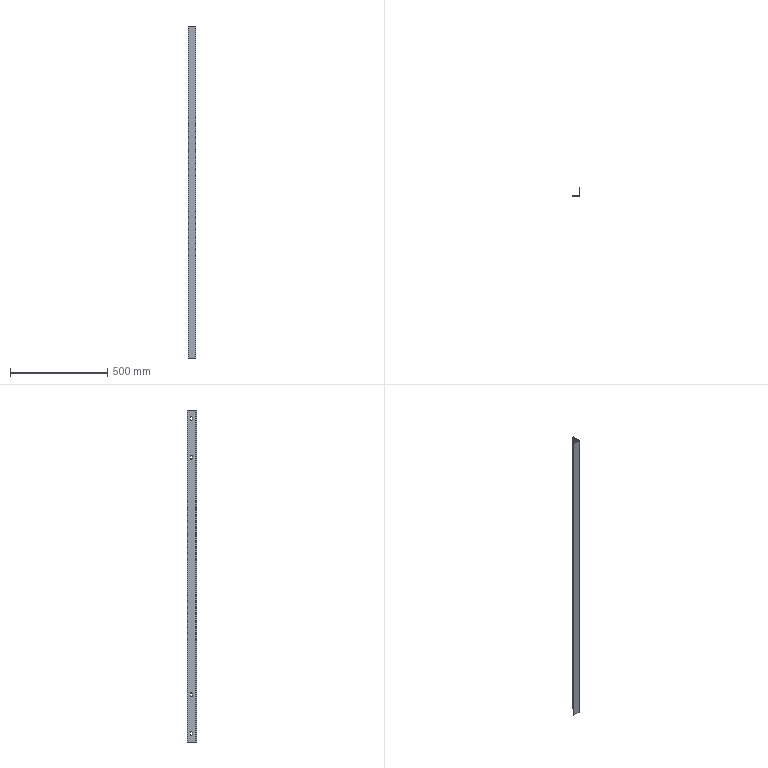Part | STEP file | SYL_0392D6J1SYL0380DJ100-519976 | 1 solid | 38 faces | box 41 x 47 x 1707 mm | volume 289245 mm3 | plane 20 | cylinder 18 | commonest cylinder face diameters 10 x16 2 x1 6 x1
STEP:
#1=CARTESIAN_POINT('',(0.,32.5,805.));
#2=VERTEX_POINT('',#1);
#3=CARTESIAN_POINT('',(-2.,32.5,805.));
#4=VERTEX_POINT('',#3);
#5=CARTESIAN_POINT('',(-2.,32.5,805.));
#6=DIRECTION('',(-1.,0.,0.));
#7=VECTOR('',#6,1000.);
#8=LINE('',#5,#7);
#9=EDGE_CURVE('',#2,#4,#8,.T.);
#10=ORIENTED_EDGE('',*,*,#9,.F.);
#11=CARTESIAN_POINT('',(0.,32.5,815.));
#12=VERTEX_POINT('',#11);
#13=CARTESIAN_POINT('',(0.,32.5,-853.5));
#14=DIRECTION('',(0.,0.,1.));
#15=VECTOR('',#14,1000.);
#16=LINE('',#13,#15);
#17=EDGE_CURVE('',#2,#12,#16,.T.);
#18=ORIENTED_EDGE('',*,*,#17,.T.);
#19=CARTESIAN_POINT('',(-2.,32.5,815.));
#20=VERTEX_POINT('',#19);
#21=CARTESIAN_POINT('',(-2.,32.5,815.));
#22=DIRECTION('',(-1.,0.,0.));
#23=VECTOR('',#22,1000.);
#24=LINE('',#21,#23);
#25=EDGE_CURVE('',#12,#20,#24,.T.);
#26=ORIENTED_EDGE('',*,*,#25,.T.);
#27=CARTESIAN_POINT('',(-2.,32.5,805.));
#28=DIRECTION('',(0.,0.,1.));
#29=VECTOR('',#28,1000.);
#30=LINE('',#27,#29);
#31=EDGE_CURVE('',#4,#20,#30,.T.);
#32=ORIENTED_EDGE('',*,*,#31,.F.);
#33=EDGE_LOOP('',(#10,#18,#26,#32));
#34=FACE_OUTER_BOUND('',#33,.T.);
#35=CARTESIAN_POINT('',(-2.,32.5,805.));
#36=DIRECTION('',(0.,1.,0.));
#37=DIRECTION('',(0.,0.,1.));
#38=AXIS2_PLACEMENT_3D('',#35,#36,#37);
#39=PLANE('',#38);
#40=ADVANCED_FACE('',(#34),#39,.F.);
#41=ORIENTED_EDGE('',*,*,#25,.F.);
#42=CARTESIAN_POINT('',(0.,27.5,820.));
#43=VERTEX_POINT('',#42);
#44=CARTESIAN_POINT('',(0.,27.5,815.));
#45=DIRECTION('',(1.,0.,0.));
#46=DIRECTION('',(0.,0.,-1.));
#47=AXIS2_PLACEMENT_3D('',#44,#45,#46);
#48=CIRCLE('',#47,5.);
#49=EDGE_CURVE('',#12,#43,#48,.T.);
#50=ORIENTED_EDGE('',*,*,#49,.T.);
#51=CARTESIAN_POINT('',(-2.,27.5,820.));
#52=VERTEX_POINT('',#51);
#53=CARTESIAN_POINT('',(-2.,27.5,820.));
#54=DIRECTION('',(-1.,0.,0.));
#55=VECTOR('',#54,1000.);
#56=LINE('',#53,#55);
#57=EDGE_CURVE('',#43,#52,#56,.T.);
#58=ORIENTED_EDGE('',*,*,#57,.T.);
#59=CARTESIAN_POINT('',(-2.,27.5,815.));
#60=DIRECTION('',(1.,0.,0.));
#61=DIRECTION('',(0.,1.,0.));
#62=AXIS2_PLACEMENT_3D('',#59,#60,#61);
#63=CIRCLE('',#62,5.);
#64=EDGE_CURVE('',#20,#52,#63,.T.);
#65=ORIENTED_EDGE('',*,*,#64,.F.);
#66=EDGE_LOOP('',(#41,#50,#58,#65));
#67=FACE_OUTER_BOUND('',#66,.T.);
#68=CARTESIAN_POINT('',(-2.,27.5,815.));
#69=DIRECTION('',(1.,0.,0.));
#70=DIRECTION('',(0.,0.,-1.));
#71=AXIS2_PLACEMENT_3D('',#68,#69,#70);
#72=CYLINDRICAL_SURFACE('',#71,5.);
#73=ADVANCED_FACE('',(#67),#72,.F.);
#74=ORIENTED_EDGE('',*,*,#57,.F.);
#75=CARTESIAN_POINT('',(0.,22.5,815.));
#76=VERTEX_POINT('',#75);
#77=CARTESIAN_POINT('',(0.,27.5,815.));
#78=DIRECTION('',(1.,0.,0.));
#79=DIRECTION('',(0.,0.,-1.));
#80=AXIS2_PLACEMENT_3D('',#77,#78,#79);
#81=CIRCLE('',#80,5.);
#82=EDGE_CURVE('',#43,#76,#81,.T.);
#83=ORIENTED_EDGE('',*,*,#82,.T.);
#84=CARTESIAN_POINT('',(-2.,22.5,815.));
#85=VERTEX_POINT('',#84);
#86=CARTESIAN_POINT('',(-2.,22.5,815.));
#87=DIRECTION('',(-1.,0.,0.));
#88=VECTOR('',#87,1000.);
#89=LINE('',#86,#88);
#90=EDGE_CURVE('',#76,#85,#89,.T.);
#91=ORIENTED_EDGE('',*,*,#90,.T.);
#92=CARTESIAN_POINT('',(-2.,27.5,815.));
#93=DIRECTION('',(1.,0.,0.));
#94=DIRECTION('',(0.,0.,1.));
#95=AXIS2_PLACEMENT_3D('',#92,#93,#94);
#96=CIRCLE('',#95,5.);
#97=EDGE_CURVE('',#52,#85,#96,.T.);
#98=ORIENTED_EDGE('',*,*,#97,.F.);
#99=EDGE_LOOP('',(#74,#83,#91,#98));
#100=FACE_OUTER_BOUND('',#99,.T.);
#101=CARTESIAN_POINT('',(-2.,27.5,815.));
#102=DIRECTION('',(1.,0.,0.));
#103=DIRECTION('',(0.,0.,-1.));
#104=AXIS2_PLACEMENT_3D('',#101,#102,#103);
#105=CYLINDRICAL_SURFACE('',#104,5.);
#106=ADVANCED_FACE('',(#100),#105,.F.);
#107=ORIENTED_EDGE('',*,*,#90,.F.);
#108=CARTESIAN_POINT('',(0.,22.5,805.));
#109=VERTEX_POINT('',#108);
#110=CARTESIAN_POINT('',(0.,22.5,-853.5));
#111=DIRECTION('',(0.,0.,-1.));
#112=VECTOR('',#111,1000.);
#113=LINE('',#110,#112);
#114=EDGE_CURVE('',#76,#109,#113,.T.);
#115=ORIENTED_EDGE('',*,*,#114,.T.);
#116=CARTESIAN_POINT('',(-2.,22.5,805.));
#117=VERTEX_POINT('',#116);
#118=CARTESIAN_POINT('',(-2.,22.5,805.));
#119=DIRECTION('',(-1.,0.,0.));
#120=VECTOR('',#119,1000.);
#121=LINE('',#118,#120);
#122=EDGE_CURVE('',#109,#117,#121,.T.);
#123=ORIENTED_EDGE('',*,*,#122,.T.);
#124=CARTESIAN_POINT('',(-2.,22.5,815.));
#125=DIRECTION('',(0.,0.,-1.));
#126=VECTOR('',#125,1000.);
#127=LINE('',#124,#126);
#128=EDGE_CURVE('',#85,#117,#127,.T.);
#129=ORIENTED_EDGE('',*,*,#128,.F.);
#130=EDGE_LOOP('',(#107,#115,#123,#129));
#131=FACE_OUTER_BOUND('',#130,.T.);
#132=CARTESIAN_POINT('',(-2.,22.5,815.));
#133=DIRECTION('',(0.,-1.,0.));
#134=DIRECTION('',(0.,0.,-1.));
#135=AXIS2_PLACEMENT_3D('',#132,#133,#134);
#136=PLANE('',#135);
#137=ADVANCED_FACE('',(#131),#136,.F.);
#138=ORIENTED_EDGE('',*,*,#122,.F.);
#139=CARTESIAN_POINT('',(0.,27.5,800.));
#140=VERTEX_POINT('',#139);
#141=CARTESIAN_POINT('',(0.,27.5,805.));
#142=DIRECTION('',(1.,0.,0.));
#143=DIRECTION('',(0.,0.,-1.));
#144=AXIS2_PLACEMENT_3D('',#141,#142,#143);
#145=CIRCLE('',#144,5.);
#146=EDGE_CURVE('',#109,#140,#145,.T.);
#147=ORIENTED_EDGE('',*,*,#146,.T.);
#148=CARTESIAN_POINT('',(-2.,27.5,800.));
#149=VERTEX_POINT('',#148);
#150=CARTESIAN_POINT('',(-2.,27.5,800.));
#151=DIRECTION('',(-1.,0.,0.));
#152=VECTOR('',#151,1000.);
#153=LINE('',#150,#152);
#154=EDGE_CURVE('',#140,#149,#153,.T.);
#155=ORIENTED_EDGE('',*,*,#154,.T.);
#156=CARTESIAN_POINT('',(-2.,27.5,805.));
#157=DIRECTION('',(1.,0.,0.));
#158=DIRECTION('',(0.,-1.,0.));
#159=AXIS2_PLACEMENT_3D('',#156,#157,#158);
#160=CIRCLE('',#159,5.);
#161=EDGE_CURVE('',#117,#149,#160,.T.);
#162=ORIENTED_EDGE('',*,*,#161,.F.);
#163=EDGE_LOOP('',(#138,#147,#155,#162));
#164=FACE_OUTER_BOUND('',#163,.T.);
#165=CARTESIAN_POINT('',(-2.,27.5,805.));
#166=DIRECTION('',(1.,0.,0.));
#167=DIRECTION('',(0.,0.,-1.));
#168=AXIS2_PLACEMENT_3D('',#165,#166,#167);
#169=CYLINDRICAL_SURFACE('',#168,5.);
#170=ADVANCED_FACE('',(#164),#169,.F.);
#171=CARTESIAN_POINT('',(0.,32.5,605.));
#172=VERTEX_POINT('',#171);
#173=CARTESIAN_POINT('',(-2.,32.5,605.));
#174=VERTEX_POINT('',#173);
#175=CARTESIAN_POINT('',(-2.,32.5,605.));
#176=DIRECTION('',(-1.,0.,0.));
#177=VECTOR('',#176,1000.);
#178=LINE('',#175,#177);
#179=EDGE_CURVE('',#172,#174,#178,.T.);
#180=ORIENTED_EDGE('',*,*,#179,.F.);
#181=CARTESIAN_POINT('',(0.,32.5,615.));
#182=VERTEX_POINT('',#181);
#183=CARTESIAN_POINT('',(0.,32.5,-853.5));
#184=DIRECTION('',(0.,0.,1.));
#185=VECTOR('',#184,1000.);
#186=LINE('',#183,#185);
#187=EDGE_CURVE('',#172,#182,#186,.T.);
#188=ORIENTED_EDGE('',*,*,#187,.T.);
#189=CARTESIAN_POINT('',(-2.,32.5,615.));
#190=VERTEX_POINT('',#189);
#191=CARTESIAN_POINT('',(-2.,32.5,615.));
#192=DIRECTION('',(-1.,0.,0.));
#193=VECTOR('',#192,1000.);
#194=LINE('',#191,#193);
#195=EDGE_CURVE('',#182,#190,#194,.T.);
#196=ORIENTED_EDGE('',*,*,#195,.T.);
#197=CARTESIAN_POINT('',(-2.,32.5,605.));
#198=DIRECTION('',(0.,0.,1.));
#199=VECTOR('',#198,1000.);
#200=LINE('',#197,#199);
#201=EDGE_CURVE('',#174,#190,#200,.T.);
#202=ORIENTED_EDGE('',*,*,#201,.F.);
#203=EDGE_LOOP('',(#180,#188,#196,#202));
#204=FACE_OUTER_BOUND('',#203,.T.);
#205=CARTESIAN_POINT('',(-2.,32.5,605.));
#206=DIRECTION('',(0.,1.,0.));
#207=DIRECTION('',(0.,0.,1.));
#208=AXIS2_PLACEMENT_3D('',#205,#206,#207);
#209=PLANE('',#208);
#210=ADVANCED_FACE('',(#204),#209,.F.);
#211=ORIENTED_EDGE('',*,*,#195,.F.);
#212=CARTESIAN_POINT('',(0.,27.5,620.));
#213=VERTEX_POINT('',#212);
#214=CARTESIAN_POINT('',(0.,27.5,615.));
#215=DIRECTION('',(1.,0.,0.));
#216=DIRECTION('',(0.,0.,-1.));
#217=AXIS2_PLACEMENT_3D('',#214,#215,#216);
#218=CIRCLE('',#217,5.);
#219=EDGE_CURVE('',#182,#213,#218,.T.);
#220=ORIENTED_EDGE('',*,*,#219,.T.);
#221=CARTESIAN_POINT('',(-2.,27.5,620.));
#222=VERTEX_POINT('',#221);
#223=CARTESIAN_POINT('',(-2.,27.5,620.));
#224=DIRECTION('',(-1.,0.,0.));
#225=VECTOR('',#224,1000.);
#226=LINE('',#223,#225);
#227=EDGE_CURVE('',#213,#222,#226,.T.);
#228=ORIENTED_EDGE('',*,*,#227,.T.);
#229=CARTESIAN_POINT('',(-2.,27.5,615.));
#230=DIRECTION('',(1.,0.,0.));
#231=DIRECTION('',(0.,1.,0.));
#232=AXIS2_PLACEMENT_3D('',#229,#230,#231);
#233=CIRCLE('',#232,5.);
#234=EDGE_CURVE('',#190,#222,#233,.T.);
#235=ORIENTED_EDGE('',*,*,#234,.F.);
#236=EDGE_LOOP('',(#211,#220,#228,#235));
#237=FACE_OUTER_BOUND('',#236,.T.);
#238=CARTESIAN_POINT('',(-2.,27.5,615.));
#239=DIRECTION('',(1.,0.,0.));
#240=DIRECTION('',(0.,0.,-1.));
#241=AXIS2_PLACEMENT_3D('',#238,#239,#240);
#242=CYLINDRICAL_SURFACE('',#241,5.);
#243=ADVANCED_FACE('',(#237),#242,.F.);
#244=ORIENTED_EDGE('',*,*,#227,.F.);
#245=CARTESIAN_POINT('',(0.,22.5,615.));
#246=VERTEX_POINT('',#245);
#247=CARTESIAN_POINT('',(0.,27.5,615.));
#248=DIRECTION('',(1.,0.,0.));
#249=DIRECTION('',(0.,0.,-1.));
#250=AXIS2_PLACEMENT_3D('',#247,#248,#249);
#251=CIRCLE('',#250,5.);
#252=EDGE_CURVE('',#213,#246,#251,.T.);
#253=ORIENTED_EDGE('',*,*,#252,.T.);
#254=CARTESIAN_POINT('',(-2.,22.5,615.));
#255=VERTEX_POINT('',#254);
#256=CARTESIAN_POINT('',(-2.,22.5,615.));
#257=DIRECTION('',(-1.,0.,0.));
#258=VECTOR('',#257,1000.);
#259=LINE('',#256,#258);
#260=EDGE_CURVE('',#246,#255,#259,.T.);
#261=ORIENTED_EDGE('',*,*,#260,.T.);
#262=CARTESIAN_POINT('',(-2.,27.5,615.));
#263=DIRECTION('',(1.,0.,0.));
#264=DIRECTION('',(0.,0.,1.));
#265=AXIS2_PLACEMENT_3D('',#262,#263,#264);
#266=CIRCLE('',#265,5.);
#267=EDGE_CURVE('',#222,#255,#266,.T.);
#268=ORIENTED_EDGE('',*,*,#267,.F.);
#269=EDGE_LOOP('',(#244,#253,#261,#268));
#270=FACE_OUTER_BOUND('',#269,.T.);
#271=CARTESIAN_POINT('',(-2.,27.5,615.));
#272=DIRECTION('',(1.,0.,0.));
#273=DIRECTION('',(0.,0.,-1.));
#274=AXIS2_PLACEMENT_3D('',#271,#272,#273);
#275=CYLINDRICAL_SURFACE('',#274,5.);
#276=ADVANCED_FACE('',(#270),#275,.F.);
#277=ORIENTED_EDGE('',*,*,#260,.F.);
#278=CARTESIAN_POINT('',(0.,22.5,605.));
#279=VERTEX_POINT('',#278);
#280=CARTESIAN_POINT('',(0.,22.5,-853.5));
#281=DIRECTION('',(0.,0.,-1.));
#282=VECTOR('',#281,1000.);
#283=LINE('',#280,#282);
#284=EDGE_CURVE('',#246,#279,#283,.T.);
#285=ORIENTED_EDGE('',*,*,#284,.T.);
#286=CARTESIAN_POINT('',(-2.,22.5,605.));
#287=VERTEX_POINT('',#286);
#288=CARTESIAN_POINT('',(-2.,22.5,605.));
#289=DIRECTION('',(-1.,0.,0.));
#290=VECTOR('',#289,1000.);
#291=LINE('',#288,#290);
#292=EDGE_CURVE('',#279,#287,#291,.T.);
#293=ORIENTED_EDGE('',*,*,#292,.T.);
#294=CARTESIAN_POINT('',(-2.,22.5,615.));
#295=DIRECTION('',(0.,0.,-1.));
#296=VECTOR('',#295,1000.);
#297=LINE('',#294,#296);
#298=EDGE_CURVE('',#255,#287,#297,.T.);
#299=ORIENTED_EDGE('',*,*,#298,.F.);
#300=EDGE_LOOP('',(#277,#285,#293,#299));
#301=FACE_OUTER_BOUND('',#300,.T.);
#302=CARTESIAN_POINT('',(-2.,22.5,615.));
#303=DIRECTION('',(0.,-1.,0.));
#304=DIRECTION('',(0.,0.,-1.));
#305=AXIS2_PLACEMENT_3D('',#302,#303,#304);
#306=PLANE('',#305);
#307=ADVANCED_FACE('',(#301),#306,.F.);
#308=ORIENTED_EDGE('',*,*,#292,.F.);
#309=CARTESIAN_POINT('',(0.,27.5,600.));
#310=VERTEX_POINT('',#309);
#311=CARTESIAN_POINT('',(0.,27.5,605.));
#312=DIRECTION('',(1.,0.,0.));
#313=DIRECTION('',(0.,0.,-1.));
#314=AXIS2_PLACEMENT_3D('',#311,#312,#313);
#315=CIRCLE('',#314,5.);
#316=EDGE_CURVE('',#279,#310,#315,.T.);
#317=ORIENTED_EDGE('',*,*,#316,.T.);
#318=CARTESIAN_POINT('',(-2.,27.5,600.));
#319=VERTEX_POINT('',#318);
#320=CARTESIAN_POINT('',(-2.,27.5,600.));
#321=DIRECTION('',(-1.,0.,0.));
#322=VECTOR('',#321,1000.);
#323=LINE('',#320,#322);
#324=EDGE_CURVE('',#310,#319,#323,.T.);
#325=ORIENTED_EDGE('',*,*,#324,.T.);
#326=CARTESIAN_POINT('',(-2.,27.5,605.));
#327=DIRECTION('',(1.,0.,0.));
#328=DIRECTION('',(0.,-1.,0.));
#329=AXIS2_PLACEMENT_3D('',#326,#327,#328);
#330=CIRCLE('',#329,5.);
#331=EDGE_CURVE('',#287,#319,#330,.T.);
#332=ORIENTED_EDGE('',*,*,#331,.F.);
#333=EDGE_LOOP('',(#308,#317,#325,#332));
#334=FACE_OUTER_BOUND('',#333,.T.);
#335=CARTESIAN_POINT('',(-2.,27.5,605.));
#336=DIRECTION('',(1.,0.,0.));
#337=DIRECTION('',(0.,0.,-1.));
#338=AXIS2_PLACEMENT_3D('',#335,#336,#337);
#339=CYLINDRICAL_SURFACE('',#338,5.);
#340=ADVANCED_FACE('',(#334),#339,.F.);
#341=CARTESIAN_POINT('',(0.,32.5,-815.));
#342=VERTEX_POINT('',#341);
#343=CARTESIAN_POINT('',(-2.,32.5,-815.));
#344=VERTEX_POINT('',#343);
#345=CARTESIAN_POINT('',(-2.,32.5,-815.));
#346=DIRECTION('',(-1.,0.,0.));
#347=VECTOR('',#346,1000.);
#348=LINE('',#345,#347);
#349=EDGE_CURVE('',#342,#344,#348,.T.);
#350=ORIENTED_EDGE('',*,*,#349,.F.);
#351=CARTESIAN_POINT('',(0.,32.5,-805.));
#352=VERTEX_POINT('',#351);
#353=CARTESIAN_POINT('',(0.,32.5,-853.5));
#354=DIRECTION('',(0.,0.,-1.));
#355=VECTOR('',#354,1000.);
#356=LINE('',#353,#355);
#357=EDGE_CURVE('',#352,#342,#356,.T.);
#358=ORIENTED_EDGE('',*,*,#357,.F.);
#359=CARTESIAN_POINT('',(-2.,32.5,-805.));
#360=VERTEX_POINT('',#359);
#361=CARTESIAN_POINT('',(-2.,32.5,-805.));
#362=DIRECTION('',(-1.,0.,0.));
#363=VECTOR('',#362,1000.);
#364=LINE('',#361,#363);
#365=EDGE_CURVE('',#352,#360,#364,.T.);
#366=ORIENTED_EDGE('',*,*,#365,.T.);
#367=CARTESIAN_POINT('',(-2.,32.5,-805.));
#368=DIRECTION('',(0.,0.,-1.));
#369=VECTOR('',#368,1000.);
#370=LINE('',#367,#369);
#371=EDGE_CURVE('',#360,#344,#370,.T.);
#372=ORIENTED_EDGE('',*,*,#371,.T.);
#373=EDGE_LOOP('',(#350,#358,#366,#372));
#374=FACE_OUTER_BOUND('',#373,.T.);
#375=CARTESIAN_POINT('',(-2.,32.5,-805.));
#376=DIRECTION('',(0.,-1.,0.));
#377=DIRECTION('',(0.,0.,-1.));
#378=AXIS2_PLACEMENT_3D('',#375,#376,#377);
#379=PLANE('',#378);
#380=ADVANCED_FACE('',(#374),#379,.T.);
#381=ORIENTED_EDGE('',*,*,#365,.F.);
#382=CARTESIAN_POINT('',(0.,27.5,-800.));
#383=VERTEX_POINT('',#382);
#384=CARTESIAN_POINT('',(0.,27.5,-805.));
#385=DIRECTION('',(1.,0.,0.));
#386=DIRECTION('',(0.,0.,-1.));
#387=AXIS2_PLACEMENT_3D('',#384,#385,#386);
#388=CIRCLE('',#387,5.);
#389=EDGE_CURVE('',#352,#383,#388,.T.);
#390=ORIENTED_EDGE('',*,*,#389,.T.);
#391=CARTESIAN_POINT('',(-2.,27.5,-800.));
#392=VERTEX_POINT('',#391);
#393=CARTESIAN_POINT('',(-2.,27.5,-800.));
#394=DIRECTION('',(-1.,0.,0.));
#395=VECTOR('',#394,1000.);
#396=LINE('',#393,#395);
#397=EDGE_CURVE('',#383,#392,#396,.T.);
#398=ORIENTED_EDGE('',*,*,#397,.T.);
#399=CARTESIAN_POINT('',(-2.,27.5,-805.));
#400=DIRECTION('',(1.,0.,0.));
#401=DIRECTION('',(0.,1.,0.));
#402=AXIS2_PLACEMENT_3D('',#399,#400,#401);
#403=CIRCLE('',#402,5.);
#404=EDGE_CURVE('',#360,#392,#403,.T.);
#405=ORIENTED_EDGE('',*,*,#404,.F.);
#406=EDGE_LOOP('',(#381,#390,#398,#405));
#407=FACE_OUTER_BOUND('',#406,.T.);
#408=CARTESIAN_POINT('',(-2.,27.5,-805.));
#409=DIRECTION('',(1.,0.,0.));
#410=DIRECTION('',(0.,0.,-1.));
#411=AXIS2_PLACEMENT_3D('',#408,#409,#410);
#412=CYLINDRICAL_SURFACE('',#411,5.);
#413=ADVANCED_FACE('',(#407),#412,.F.);
#414=ORIENTED_EDGE('',*,*,#397,.F.);
#415=CARTESIAN_POINT('',(0.,22.5,-805.));
#416=VERTEX_POINT('',#415);
#417=CARTESIAN_POINT('',(0.,27.5,-805.));
#418=DIRECTION('',(1.,0.,0.));
#419=DIRECTION('',(0.,0.,-1.));
#420=AXIS2_PLACEMENT_3D('',#417,#418,#419);
#421=CIRCLE('',#420,5.);
#422=EDGE_CURVE('',#383,#416,#421,.T.);
#423=ORIENTED_EDGE('',*,*,#422,.T.);
#424=CARTESIAN_POINT('',(-2.,22.5,-805.));
#425=VERTEX_POINT('',#424);
#426=CARTESIAN_POINT('',(-2.,22.5,-805.));
#427=DIRECTION('',(-1.,0.,0.));
#428=VECTOR('',#427,1000.);
#429=LINE('',#426,#428);
#430=EDGE_CURVE('',#416,#425,#429,.T.);
#431=ORIENTED_EDGE('',*,*,#430,.T.);
#432=CARTESIAN_POINT('',(-2.,27.5,-805.));
#433=DIRECTION('',(1.,0.,0.));
#434=DIRECTION('',(0.,0.,1.));
#435=AXIS2_PLACEMENT_3D('',#432,#433,#434);
#436=CIRCLE('',#435,5.);
#437=EDGE_CURVE('',#392,#425,#436,.T.);
#438=ORIENTED_EDGE('',*,*,#437,.F.);
#439=EDGE_LOOP('',(#414,#423,#431,#438));
#440=FACE_OUTER_BOUND('',#439,.T.);
#441=CARTESIAN_POINT('',(-2.,27.5,-805.));
#442=DIRECTION('',(1.,0.,0.));
#443=DIRECTION('',(0.,0.,-1.));
#444=AXIS2_PLACEMENT_3D('',#441,#442,#443);
#445=CYLINDRICAL_SURFACE('',#444,5.);
#446=ADVANCED_FACE('',(#440),#445,.F.);
#447=ORIENTED_EDGE('',*,*,#430,.F.);
#448=CARTESIAN_POINT('',(0.,22.5,-815.));
#449=VERTEX_POINT('',#448);
#450=CARTESIAN_POINT('',(0.,22.5,-853.5));
#451=DIRECTION('',(0.,0.,1.));
#452=VECTOR('',#451,1000.);
#453=LINE('',#450,#452);
#454=EDGE_CURVE('',#449,#416,#453,.T.);
#455=ORIENTED_EDGE('',*,*,#454,.F.);
#456=CARTESIAN_POINT('',(-2.,22.5,-815.));
#457=VERTEX_POINT('',#456);
#458=CARTESIAN_POINT('',(-2.,22.5,-815.));
#459=DIRECTION('',(-1.,0.,0.));
#460=VECTOR('',#459,1000.);
#461=LINE('',#458,#460);
#462=EDGE_CURVE('',#449,#457,#461,.T.);
#463=ORIENTED_EDGE('',*,*,#462,.T.);
#464=CARTESIAN_POINT('',(-2.,22.5,-815.));
#465=DIRECTION('',(0.,0.,1.));
#466=VECTOR('',#465,1000.);
#467=LINE('',#464,#466);
#468=EDGE_CURVE('',#457,#425,#467,.T.);
#469=ORIENTED_EDGE('',*,*,#468,.T.);
#470=EDGE_LOOP('',(#447,#455,#463,#469));
#471=FACE_OUTER_BOUND('',#470,.T.);
#472=CARTESIAN_POINT('',(-2.,22.5,-815.));
#473=DIRECTION('',(0.,1.,0.));
#474=DIRECTION('',(0.,0.,1.));
#475=AXIS2_PLACEMENT_3D('',#472,#473,#474);
#476=PLANE('',#475);
#477=ADVANCED_FACE('',(#471),#476,.T.);
#478=ORIENTED_EDGE('',*,*,#462,.F.);
#479=CARTESIAN_POINT('',(0.,27.5,-820.));
#480=VERTEX_POINT('',#479);
#481=CARTESIAN_POINT('',(0.,27.5,-815.));
#482=DIRECTION('',(1.,0.,0.));
#483=DIRECTION('',(0.,0.,-1.));
#484=AXIS2_PLACEMENT_3D('',#481,#482,#483);
#485=CIRCLE('',#484,5.);
#486=EDGE_CURVE('',#449,#480,#485,.T.);
#487=ORIENTED_EDGE('',*,*,#486,.T.);
#488=CARTESIAN_POINT('',(-2.,27.5,-820.));
#489=VERTEX_POINT('',#488);
#490=CARTESIAN_POINT('',(-2.,27.5,-820.));
#491=DIRECTION('',(-1.,0.,0.));
#492=VECTOR('',#491,1000.);
#493=LINE('',#490,#492);
#494=EDGE_CURVE('',#480,#489,#493,.T.);
#495=ORIENTED_EDGE('',*,*,#494,.T.);
#496=CARTESIAN_POINT('',(-2.,27.5,-815.));
#497=DIRECTION('',(1.,0.,0.));
#498=DIRECTION('',(0.,-1.,0.));
#499=AXIS2_PLACEMENT_3D('',#496,#497,#498);
#500=CIRCLE('',#499,5.);
#501=EDGE_CURVE('',#457,#489,#500,.T.);
#502=ORIENTED_EDGE('',*,*,#501,.F.);
#503=EDGE_LOOP('',(#478,#487,#495,#502));
#504=FACE_OUTER_BOUND('',#503,.T.);
#505=CARTESIAN_POINT('',(-2.,27.5,-815.));
#506=DIRECTION('',(1.,0.,0.));
#507=DIRECTION('',(0.,0.,-1.));
#508=AXIS2_PLACEMENT_3D('',#505,#506,#507);
#509=CYLINDRICAL_SURFACE('',#508,5.);
#510=ADVANCED_FACE('',(#504),#509,.F.);
#511=CARTESIAN_POINT('',(0.,32.5,-615.));
#512=VERTEX_POINT('',#511);
#513=CARTESIAN_POINT('',(-2.,32.5,-615.));
#514=VERTEX_POINT('',#513);
#515=CARTESIAN_POINT('',(-2.,32.5,-615.));
#516=DIRECTION('',(-1.,0.,0.));
#517=VECTOR('',#516,1000.);
#518=LINE('',#515,#517);
#519=EDGE_CURVE('',#512,#514,#518,.T.);
#520=ORIENTED_EDGE('',*,*,#519,.F.);
#521=CARTESIAN_POINT('',(0.,32.5,-605.));
#522=VERTEX_POINT('',#521);
#523=CARTESIAN_POINT('',(0.,32.5,-853.5));
#524=DIRECTION('',(0.,0.,-1.));
#525=VECTOR('',#524,1000.);
#526=LINE('',#523,#525);
#527=EDGE_CURVE('',#522,#512,#526,.T.);
#528=ORIENTED_EDGE('',*,*,#527,.F.);
#529=CARTESIAN_POINT('',(-2.,32.5,-605.));
#530=VERTEX_POINT('',#529);
#531=CARTESIAN_POINT('',(-2.,32.5,-605.));
#532=DIRECTION('',(-1.,0.,0.));
#533=VECTOR('',#532,1000.);
#534=LINE('',#531,#533);
#535=EDGE_CURVE('',#522,#530,#534,.T.);
#536=ORIENTED_EDGE('',*,*,#535,.T.);
#537=CARTESIAN_POINT('',(-2.,32.5,-605.));
#538=DIRECTION('',(0.,0.,-1.));
#539=VECTOR('',#538,1000.);
#540=LINE('',#537,#539);
#541=EDGE_CURVE('',#530,#514,#540,.T.);
#542=ORIENTED_EDGE('',*,*,#541,.T.);
#543=EDGE_LOOP('',(#520,#528,#536,#542));
#544=FACE_OUTER_BOUND('',#543,.T.);
#545=CARTESIAN_POINT('',(-2.,32.5,-605.));
#546=DIRECTION('',(0.,-1.,0.));
#547=DIRECTION('',(0.,0.,-1.));
#548=AXIS2_PLACEMENT_3D('',#545,#546,#547);
#549=PLANE('',#548);
#550=ADVANCED_FACE('',(#544),#549,.T.);
#551=ORIENTED_EDGE('',*,*,#535,.F.);
#552=CARTESIAN_POINT('',(0.,27.5,-600.));
#553=VERTEX_POINT('',#552);
#554=CARTESIAN_POINT('',(0.,27.5,-605.));
#555=DIRECTION('',(1.,0.,0.));
#556=DIRECTION('',(0.,0.,-1.));
#557=AXIS2_PLACEMENT_3D('',#554,#555,#556);
#558=CIRCLE('',#557,5.);
#559=EDGE_CURVE('',#522,#553,#558,.T.);
#560=ORIENTED_EDGE('',*,*,#559,.T.);
#561=CARTESIAN_POINT('',(-2.,27.5,-600.));
#562=VERTEX_POINT('',#561);
#563=CARTESIAN_POINT('',(-2.,27.5,-600.));
#564=DIRECTION('',(-1.,0.,0.));
#565=VECTOR('',#564,1000.);
#566=LINE('',#563,#565);
#567=EDGE_CURVE('',#553,#562,#566,.T.);
#568=ORIENTED_EDGE('',*,*,#567,.T.);
#569=CARTESIAN_POINT('',(-2.,27.5,-605.));
#570=DIRECTION('',(1.,0.,0.));
#571=DIRECTION('',(0.,1.,0.));
#572=AXIS2_PLACEMENT_3D('',#569,#570,#571);
#573=CIRCLE('',#572,5.);
#574=EDGE_CURVE('',#530,#562,#573,.T.);
#575=ORIENTED_EDGE('',*,*,#574,.F.);
#576=EDGE_LOOP('',(#551,#560,#568,#575));
#577=FACE_OUTER_BOUND('',#576,.T.);
#578=CARTESIAN_POINT('',(-2.,27.5,-605.));
#579=DIRECTION('',(1.,0.,0.));
#580=DIRECTION('',(0.,0.,-1.));
#581=AXIS2_PLACEMENT_3D('',#578,#579,#580);
#582=CYLINDRICAL_SURFACE('',#581,5.);
#583=ADVANCED_FACE('',(#577),#582,.F.);
#584=ORIENTED_EDGE('',*,*,#567,.F.);
#585=CARTESIAN_POINT('',(0.,22.5,-605.));
#586=VERTEX_POINT('',#585);
#587=CARTESIAN_POINT('',(0.,27.5,-605.));
#588=DIRECTION('',(1.,0.,0.));
#589=DIRECTION('',(0.,0.,-1.));
#590=AXIS2_PLACEMENT_3D('',#587,#588,#589);
#591=CIRCLE('',#590,5.);
#592=EDGE_CURVE('',#553,#586,#591,.T.);
#593=ORIENTED_EDGE('',*,*,#592,.T.);
#594=CARTESIAN_POINT('',(-2.,22.5,-605.));
#595=VERTEX_POINT('',#594);
#596=CARTESIAN_POINT('',(-2.,22.5,-605.));
#597=DIRECTION('',(-1.,0.,0.));
#598=VECTOR('',#597,1000.);
#599=LINE('',#596,#598);
#600=EDGE_CURVE('',#586,#595,#599,.T.);
#601=ORIENTED_EDGE('',*,*,#600,.T.);
#602=CARTESIAN_POINT('',(-2.,27.5,-605.));
#603=DIRECTION('',(1.,0.,0.));
#604=DIRECTION('',(0.,0.,1.));
#605=AXIS2_PLACEMENT_3D('',#602,#603,#604);
#606=CIRCLE('',#605,5.);
#607=EDGE_CURVE('',#562,#595,#606,.T.);
#608=ORIENTED_EDGE('',*,*,#607,.F.);
#609=EDGE_LOOP('',(#584,#593,#601,#608));
#610=FACE_OUTER_BOUND('',#609,.T.);
#611=CARTESIAN_POINT('',(-2.,27.5,-605.));
#612=DIRECTION('',(1.,0.,0.));
#613=DIRECTION('',(0.,0.,-1.));
#614=AXIS2_PLACEMENT_3D('',#611,#612,#613);
#615=CYLINDRICAL_SURFACE('',#614,5.);
#616=ADVANCED_FACE('',(#610),#615,.F.);
#617=ORIENTED_EDGE('',*,*,#600,.F.);
#618=CARTESIAN_POINT('',(0.,22.5,-615.));
#619=VERTEX_POINT('',#618);
#620=CARTESIAN_POINT('',(0.,22.5,-853.5));
#621=DIRECTION('',(0.,0.,1.));
#622=VECTOR('',#621,1000.);
#623=LINE('',#620,#622);
#624=EDGE_CURVE('',#619,#586,#623,.T.);
#625=ORIENTED_EDGE('',*,*,#624,.F.);
#626=CARTESIAN_POINT('',(-2.,22.5,-615.));
#627=VERTEX_POINT('',#626);
#628=CARTESIAN_POINT('',(-2.,22.5,-615.));
#629=DIRECTION('',(-1.,0.,0.));
#630=VECTOR('',#629,1000.);
#631=LINE('',#628,#630);
#632=EDGE_CURVE('',#619,#627,#631,.T.);
#633=ORIENTED_EDGE('',*,*,#632,.T.);
#634=CARTESIAN_POINT('',(-2.,22.5,-615.));
#635=DIRECTION('',(0.,0.,1.));
#636=VECTOR('',#635,1000.);
#637=LINE('',#634,#636);
#638=EDGE_CURVE('',#627,#595,#637,.T.);
#639=ORIENTED_EDGE('',*,*,#638,.T.);
#640=EDGE_LOOP('',(#617,#625,#633,#639));
#641=FACE_OUTER_BOUND('',#640,.T.);
#642=CARTESIAN_POINT('',(-2.,22.5,-615.));
#643=DIRECTION('',(0.,1.,0.));
#644=DIRECTION('',(0.,0.,1.));
#645=AXIS2_PLACEMENT_3D('',#642,#643,#644);
#646=PLANE('',#645);
#647=ADVANCED_FACE('',(#641),#646,.T.);
#648=ORIENTED_EDGE('',*,*,#632,.F.);
#649=CARTESIAN_POINT('',(0.,27.5,-620.));
#650=VERTEX_POINT('',#649);
#651=CARTESIAN_POINT('',(0.,27.5,-615.));
#652=DIRECTION('',(1.,0.,0.));
#653=DIRECTION('',(0.,0.,-1.));
#654=AXIS2_PLACEMENT_3D('',#651,#652,#653);
#655=CIRCLE('',#654,5.);
#656=EDGE_CURVE('',#619,#650,#655,.T.);
#657=ORIENTED_EDGE('',*,*,#656,.T.);
#658=CARTESIAN_POINT('',(-2.,27.5,-620.));
#659=VERTEX_POINT('',#658);
#660=CARTESIAN_POINT('',(-2.,27.5,-620.));
#661=DIRECTION('',(-1.,0.,0.));
#662=VECTOR('',#661,1000.);
#663=LINE('',#660,#662);
#664=EDGE_CURVE('',#650,#659,#663,.T.);
#665=ORIENTED_EDGE('',*,*,#664,.T.);
#666=CARTESIAN_POINT('',(-2.,27.5,-615.));
#667=DIRECTION('',(1.,0.,0.));
#668=DIRECTION('',(0.,-1.,0.));
#669=AXIS2_PLACEMENT_3D('',#666,#667,#668);
#670=CIRCLE('',#669,5.);
#671=EDGE_CURVE('',#627,#659,#670,.T.);
#672=ORIENTED_EDGE('',*,*,#671,.F.);
#673=EDGE_LOOP('',(#648,#657,#665,#672));
#674=FACE_OUTER_BOUND('',#673,.T.);
#675=CARTESIAN_POINT('',(-2.,27.5,-615.));
#676=DIRECTION('',(1.,0.,0.));
#677=DIRECTION('',(0.,0.,-1.));
#678=AXIS2_PLACEMENT_3D('',#675,#676,#677);
#679=CYLINDRICAL_SURFACE('',#678,5.);
#680=ADVANCED_FACE('',(#674),#679,.F.);
#681=CARTESIAN_POINT('',(-41.,0.,-853.5));
#682=VERTEX_POINT('',#681);
#683=CARTESIAN_POINT('',(-41.,2.,-853.5));
#684=VERTEX_POINT('',#683);
#685=CARTESIAN_POINT('',(-41.,2.,-853.5));
#686=DIRECTION('',(0.,1.,0.));
#687=VECTOR('',#686,1000.);
#688=LINE('',#685,#687);
#689=EDGE_CURVE('',#682,#684,#688,.T.);
#690=ORIENTED_EDGE('',*,*,#689,.F.);
#691=CARTESIAN_POINT('',(-41.,0.,853.5));
#692=VERTEX_POINT('',#691);
#693=CARTESIAN_POINT('',(-41.,0.,-853.5));
#694=DIRECTION('',(0.,0.,-1.));
#695=VECTOR('',#694,1000.);
#696=LINE('',#693,#695);
#697=EDGE_CURVE('',#692,#682,#696,.T.);
#698=ORIENTED_EDGE('',*,*,#697,.F.);
#699=CARTESIAN_POINT('',(-41.,2.,853.5));
#700=VERTEX_POINT('',#699);
#701=CARTESIAN_POINT('',(-41.,2.,853.5));
#702=DIRECTION('',(0.,1.,0.));
#703=VECTOR('',#702,1000.);
#704=LINE('',#701,#703);
#705=EDGE_CURVE('',#692,#700,#704,.T.);
#706=ORIENTED_EDGE('',*,*,#705,.T.);
#707=CARTESIAN_POINT('',(-41.,2.,853.5));
#708=DIRECTION('',(0.,0.,-1.));
#709=VECTOR('',#708,1000.);
#710=LINE('',#707,#709);
#711=EDGE_CURVE('',#700,#684,#710,.T.);
#712=ORIENTED_EDGE('',*,*,#711,.T.);
#713=EDGE_LOOP('',(#690,#698,#706,#712));
#714=FACE_OUTER_BOUND('',#713,.T.);
#715=CARTESIAN_POINT('',(-41.,2.,853.5));
#716=DIRECTION('',(-1.,0.,0.));
#717=DIRECTION('',(0.,0.,-1.));
#718=AXIS2_PLACEMENT_3D('',#715,#716,#717);
#719=PLANE('',#718);
#720=ADVANCED_FACE('',(#714),#719,.T.);
#721=ORIENTED_EDGE('',*,*,#705,.F.);
#722=CARTESIAN_POINT('',(-3.,0.,853.5));
#723=VERTEX_POINT('',#722);
#724=CARTESIAN_POINT('',(-41.,0.,853.5));
#725=DIRECTION('',(-1.,0.,0.));
#726=VECTOR('',#725,1000.);
#727=LINE('',#724,#726);
#728=EDGE_CURVE('',#723,#692,#727,.T.);
#729=ORIENTED_EDGE('',*,*,#728,.F.);
#730=CARTESIAN_POINT('',(-3.,2.,853.5));
#731=VERTEX_POINT('',#730);
#732=CARTESIAN_POINT('',(-3.,2.,853.5));
#733=DIRECTION('',(0.,1.,0.));
#734=VECTOR('',#733,1000.);
#735=LINE('',#732,#734);
#736=EDGE_CURVE('',#723,#731,#735,.T.);
#737=ORIENTED_EDGE('',*,*,#736,.T.);
#738=CARTESIAN_POINT('',(-3.,2.,853.5));
#739=DIRECTION('',(-1.,0.,0.));
#740=VECTOR('',#739,1000.);
#741=LINE('',#738,#740);
#742=EDGE_CURVE('',#731,#700,#741,.T.);
#743=ORIENTED_EDGE('',*,*,#742,.T.);
#744=EDGE_LOOP('',(#721,#729,#737,#743));
#745=FACE_OUTER_BOUND('',#744,.T.);
#746=CARTESIAN_POINT('',(-3.,2.,853.5));
#747=DIRECTION('',(0.,0.,1.));
#748=DIRECTION('',(-1.,0.,0.));
#749=AXIS2_PLACEMENT_3D('',#746,#747,#748);
#750=PLANE('',#749);
#751=ADVANCED_FACE('',(#745),#750,.T.);
#752=ORIENTED_EDGE('',*,*,#736,.F.);
#753=CARTESIAN_POINT('',(0.,3.,853.5));
#754=VERTEX_POINT('',#753);
#755=CARTESIAN_POINT('',(-3.,3.,853.5));
#756=DIRECTION('',(0.,0.,-1.));
#757=DIRECTION('',(-1.,0.,0.));
#758=AXIS2_PLACEMENT_3D('',#755,#756,#757);
#759=CIRCLE('',#758,3.);
#760=EDGE_CURVE('',#754,#723,#759,.T.);
#761=ORIENTED_EDGE('',*,*,#760,.F.);
#762=CARTESIAN_POINT('',(-2.,3.,853.5));
#763=VERTEX_POINT('',#762);
#764=CARTESIAN_POINT('',(-2.,3.,853.5));
#765=DIRECTION('',(-1.,0.,0.));
#766=VECTOR('',#765,1000.);
#767=LINE('',#764,#766);
#768=EDGE_CURVE('',#754,#763,#767,.T.);
#769=ORIENTED_EDGE('',*,*,#768,.T.);
#770=CARTESIAN_POINT('',(-3.,3.,853.5));
#771=DIRECTION('',(0.,0.,-1.));
#772=DIRECTION('',(1.,0.,0.));
#773=AXIS2_PLACEMENT_3D('',#770,#771,#772);
#774=CIRCLE('',#773,1.);
#775=EDGE_CURVE('',#763,#731,#774,.T.);
#776=ORIENTED_EDGE('',*,*,#775,.T.);
#777=EDGE_LOOP('',(#752,#761,#769,#776));
#778=FACE_OUTER_BOUND('',#777,.T.);
#779=CARTESIAN_POINT('',(-3.,3.,853.5));
#780=DIRECTION('',(0.,0.,1.));
#781=DIRECTION('',(1.,0.,0.));
#782=AXIS2_PLACEMENT_3D('',#779,#780,#781);
#783=PLANE('',#782);
#784=ADVANCED_FACE('',(#778),#783,.T.);
#785=ORIENTED_EDGE('',*,*,#768,.F.);
#786=CARTESIAN_POINT('',(0.,47.,853.5));
#787=VERTEX_POINT('',#786);
#788=CARTESIAN_POINT('',(0.,0.,853.5));
#789=DIRECTION('',(0.,-1.,0.));
#790=VECTOR('',#789,1000.);
#791=LINE('',#788,#790);
#792=EDGE_CURVE('',#787,#754,#791,.T.);
#793=ORIENTED_EDGE('',*,*,#792,.F.);
#794=CARTESIAN_POINT('',(-2.,47.,853.5));
#795=VERTEX_POINT('',#794);
#796=CARTESIAN_POINT('',(-2.,47.,853.5));
#797=DIRECTION('',(-1.,0.,0.));
#798=VECTOR('',#797,1000.);
#799=LINE('',#796,#798);
#800=EDGE_CURVE('',#787,#795,#799,.T.);
#801=ORIENTED_EDGE('',*,*,#800,.T.);
#802=CARTESIAN_POINT('',(-2.,47.,853.5));
#803=DIRECTION('',(0.,-1.,0.));
#804=VECTOR('',#803,1000.);
#805=LINE('',#802,#804);
#806=EDGE_CURVE('',#795,#763,#805,.T.);
#807=ORIENTED_EDGE('',*,*,#806,.T.);
#808=EDGE_LOOP('',(#785,#793,#801,#807));
#809=FACE_OUTER_BOUND('',#808,.T.);
#810=CARTESIAN_POINT('',(-2.,47.,853.5));
#811=DIRECTION('',(0.,0.,1.));
#812=DIRECTION('',(0.,-1.,0.));
#813=AXIS2_PLACEMENT_3D('',#810,#811,#812);
#814=PLANE('',#813);
#815=ADVANCED_FACE('',(#809),#814,.T.);
#816=ORIENTED_EDGE('',*,*,#800,.F.);
#817=CARTESIAN_POINT('',(0.,47.,-853.5));
#818=VERTEX_POINT('',#817);
#819=CARTESIAN_POINT('',(0.,47.,-853.5));
#820=DIRECTION('',(0.,0.,-1.));
#821=VECTOR('',#820,1000.);
#822=LINE('',#819,#821);
#823=EDGE_CURVE('',#787,#818,#822,.T.);
#824=ORIENTED_EDGE('',*,*,#823,.T.);
#825=CARTESIAN_POINT('',(-2.,47.,-853.5));
#826=VERTEX_POINT('',#825);
#827=CARTESIAN_POINT('',(-2.,47.,-853.5));
#828=DIRECTION('',(-1.,0.,0.));
#829=VECTOR('',#828,1000.);
#830=LINE('',#827,#829);
#831=EDGE_CURVE('',#818,#826,#830,.T.);
#832=ORIENTED_EDGE('',*,*,#831,.T.);
#833=CARTESIAN_POINT('',(-2.,47.,853.5));
#834=DIRECTION('',(0.,0.,-1.));
#835=VECTOR('',#834,1000.);
#836=LINE('',#833,#835);
#837=EDGE_CURVE('',#795,#826,#836,.T.);
#838=ORIENTED_EDGE('',*,*,#837,.F.);
#839=EDGE_LOOP('',(#816,#824,#832,#838));
#840=FACE_OUTER_BOUND('',#839,.T.);
#841=CARTESIAN_POINT('',(-2.,47.,853.5));
#842=DIRECTION('',(0.,-1.,0.));
#843=DIRECTION('',(0.,0.,-1.));
#844=AXIS2_PLACEMENT_3D('',#841,#842,#843);
#845=PLANE('',#844);
#846=ADVANCED_FACE('',(#840),#845,.F.);
#847=ORIENTED_EDGE('',*,*,#831,.F.);
#848=CARTESIAN_POINT('',(0.,3.,-853.5));
#849=VERTEX_POINT('',#848);
#850=CARTESIAN_POINT('',(0.,0.,-853.5));
#851=DIRECTION('',(0.,-1.,0.));
#852=VECTOR('',#851,1000.);
#853=LINE('',#850,#852);
#854=EDGE_CURVE('',#818,#849,#853,.T.);
#855=ORIENTED_EDGE('',*,*,#854,.T.);
#856=CARTESIAN_POINT('',(-2.,3.,-853.5));
#857=VERTEX_POINT('',#856);
#858=CARTESIAN_POINT('',(-2.,3.,-853.5));
#859=DIRECTION('',(-1.,0.,0.));
#860=VECTOR('',#859,1000.);
#861=LINE('',#858,#860);
#862=EDGE_CURVE('',#849,#857,#861,.T.);
#863=ORIENTED_EDGE('',*,*,#862,.T.);
#864=CARTESIAN_POINT('',(-2.,47.,-853.5));
#865=DIRECTION('',(0.,-1.,0.));
#866=VECTOR('',#865,1000.);
#867=LINE('',#864,#866);
#868=EDGE_CURVE('',#826,#857,#867,.T.);
#869=ORIENTED_EDGE('',*,*,#868,.F.);
#870=EDGE_LOOP('',(#847,#855,#863,#869));
#871=FACE_OUTER_BOUND('',#870,.T.);
#872=CARTESIAN_POINT('',(-2.,47.,-853.5));
#873=DIRECTION('',(0.,0.,1.));
#874=DIRECTION('',(0.,-1.,0.));
#875=AXIS2_PLACEMENT_3D('',#872,#873,#874);
#876=PLANE('',#875);
#877=ADVANCED_FACE('',(#871),#876,.F.);
#878=ORIENTED_EDGE('',*,*,#862,.F.);
#879=CARTESIAN_POINT('',(-3.,0.,-853.5));
#880=VERTEX_POINT('',#879);
#881=CARTESIAN_POINT('',(-3.,3.,-853.5));
#882=DIRECTION('',(0.,0.,1.));
#883=DIRECTION('',(-1.,0.,0.));
#884=AXIS2_PLACEMENT_3D('',#881,#882,#883);
#885=CIRCLE('',#884,3.);
#886=EDGE_CURVE('',#880,#849,#885,.T.);
#887=ORIENTED_EDGE('',*,*,#886,.F.);
#888=CARTESIAN_POINT('',(-3.,2.,-853.5));
#889=VERTEX_POINT('',#888);
#890=CARTESIAN_POINT('',(-3.,2.,-853.5));
#891=DIRECTION('',(0.,1.,0.));
#892=VECTOR('',#891,1000.);
#893=LINE('',#890,#892);
#894=EDGE_CURVE('',#880,#889,#893,.T.);
#895=ORIENTED_EDGE('',*,*,#894,.T.);
#896=CARTESIAN_POINT('',(-3.,3.,-853.5));
#897=DIRECTION('',(0.,0.,1.));
#898=DIRECTION('',(0.,-1.,0.));
#899=AXIS2_PLACEMENT_3D('',#896,#897,#898);
#900=CIRCLE('',#899,1.);
#901=EDGE_CURVE('',#889,#857,#900,.T.);
#902=ORIENTED_EDGE('',*,*,#901,.T.);
#903=EDGE_LOOP('',(#878,#887,#895,#902));
#904=FACE_OUTER_BOUND('',#903,.T.);
#905=CARTESIAN_POINT('',(-3.,3.,-853.5));
#906=DIRECTION('',(0.,0.,-1.));
#907=DIRECTION('',(-1.,0.,0.));
#908=AXIS2_PLACEMENT_3D('',#905,#906,#907);
#909=PLANE('',#908);
#910=ADVANCED_FACE('',(#904),#909,.T.);
#911=CARTESIAN_POINT('',(0.,27.5,-615.));
#912=DIRECTION('',(1.,0.,0.));
#913=DIRECTION('',(0.,0.,-1.));
#914=AXIS2_PLACEMENT_3D('',#911,#912,#913);
#915=CIRCLE('',#914,5.);
#916=EDGE_CURVE('',#650,#512,#915,.T.);
#917=ORIENTED_EDGE('',*,*,#916,.T.);
#918=ORIENTED_EDGE('',*,*,#519,.T.);
#919=CARTESIAN_POINT('',(-2.,27.5,-615.));
#920=DIRECTION('',(1.,0.,0.));
#921=DIRECTION('',(0.,0.,-1.));
#922=AXIS2_PLACEMENT_3D('',#919,#920,#921);
#923=CIRCLE('',#922,5.);
#924=EDGE_CURVE('',#659,#514,#923,.T.);
#925=ORIENTED_EDGE('',*,*,#924,.F.);
#926=ORIENTED_EDGE('',*,*,#664,.F.);
#927=EDGE_LOOP('',(#917,#918,#925,#926));
#928=FACE_OUTER_BOUND('',#927,.T.);
#929=CARTESIAN_POINT('',(-2.,27.5,-615.));
#930=DIRECTION('',(1.,0.,0.));
#931=DIRECTION('',(0.,0.,-1.));
#932=AXIS2_PLACEMENT_3D('',#929,#930,#931);
#933=CYLINDRICAL_SURFACE('',#932,5.);
#934=ADVANCED_FACE('',(#928),#933,.F.);
#935=CARTESIAN_POINT('',(0.,27.5,-815.));
#936=DIRECTION('',(1.,0.,0.));
#937=DIRECTION('',(0.,0.,-1.));
#938=AXIS2_PLACEMENT_3D('',#935,#936,#937);
#939=CIRCLE('',#938,5.);
#940=EDGE_CURVE('',#480,#342,#939,.T.);
#941=ORIENTED_EDGE('',*,*,#940,.T.);
#942=ORIENTED_EDGE('',*,*,#349,.T.);
#943=CARTESIAN_POINT('',(-2.,27.5,-815.));
#944=DIRECTION('',(1.,0.,0.));
#945=DIRECTION('',(0.,0.,-1.));
#946=AXIS2_PLACEMENT_3D('',#943,#944,#945);
#947=CIRCLE('',#946,5.);
#948=EDGE_CURVE('',#489,#344,#947,.T.);
#949=ORIENTED_EDGE('',*,*,#948,.F.);
#950=ORIENTED_EDGE('',*,*,#494,.F.);
#951=EDGE_LOOP('',(#941,#942,#949,#950));
#952=FACE_OUTER_BOUND('',#951,.T.);
#953=CARTESIAN_POINT('',(-2.,27.5,-815.));
#954=DIRECTION('',(1.,0.,0.));
#955=DIRECTION('',(0.,0.,-1.));
#956=AXIS2_PLACEMENT_3D('',#953,#954,#955);
#957=CYLINDRICAL_SURFACE('',#956,5.);
#958=ADVANCED_FACE('',(#952),#957,.F.);
#959=CARTESIAN_POINT('',(0.,27.5,605.));
#960=DIRECTION('',(1.,0.,0.));
#961=DIRECTION('',(0.,0.,-1.));
#962=AXIS2_PLACEMENT_3D('',#959,#960,#961);
#963=CIRCLE('',#962,5.);
#964=EDGE_CURVE('',#310,#172,#963,.T.);
#965=ORIENTED_EDGE('',*,*,#964,.T.);
#966=ORIENTED_EDGE('',*,*,#179,.T.);
#967=CARTESIAN_POINT('',(-2.,27.5,605.));
#968=DIRECTION('',(1.,0.,0.));
#969=DIRECTION('',(0.,0.,-1.));
#970=AXIS2_PLACEMENT_3D('',#967,#968,#969);
#971=CIRCLE('',#970,5.);
#972=EDGE_CURVE('',#319,#174,#971,.T.);
#973=ORIENTED_EDGE('',*,*,#972,.F.);
#974=ORIENTED_EDGE('',*,*,#324,.F.);
#975=EDGE_LOOP('',(#965,#966,#973,#974));
#976=FACE_OUTER_BOUND('',#975,.T.);
#977=CARTESIAN_POINT('',(-2.,27.5,605.));
#978=DIRECTION('',(1.,0.,0.));
#979=DIRECTION('',(0.,0.,-1.));
#980=AXIS2_PLACEMENT_3D('',#977,#978,#979);
#981=CYLINDRICAL_SURFACE('',#980,5.);
#982=ADVANCED_FACE('',(#976),#981,.F.);
#983=CARTESIAN_POINT('',(0.,27.5,805.));
#984=DIRECTION('',(1.,0.,0.));
#985=DIRECTION('',(0.,0.,-1.));
#986=AXIS2_PLACEMENT_3D('',#983,#984,#985);
#987=CIRCLE('',#986,5.);
#988=EDGE_CURVE('',#140,#2,#987,.T.);
#989=ORIENTED_EDGE('',*,*,#988,.T.);
#990=ORIENTED_EDGE('',*,*,#9,.T.);
#991=CARTESIAN_POINT('',(-2.,27.5,805.));
#992=DIRECTION('',(1.,0.,0.));
#993=DIRECTION('',(0.,0.,-1.));
#994=AXIS2_PLACEMENT_3D('',#991,#992,#993);
#995=CIRCLE('',#994,5.);
#996=EDGE_CURVE('',#149,#4,#995,.T.);
#997=ORIENTED_EDGE('',*,*,#996,.F.);
#998=ORIENTED_EDGE('',*,*,#154,.F.);
#999=EDGE_LOOP('',(#989,#990,#997,#998));
#1000=FACE_OUTER_BOUND('',#999,.T.);
#1001=CARTESIAN_POINT('',(-2.,27.5,805.));
#1002=DIRECTION('',(1.,0.,0.));
#1003=DIRECTION('',(0.,0.,-1.));
#1004=AXIS2_PLACEMENT_3D('',#1001,#1002,#1003);
#1005=CYLINDRICAL_SURFACE('',#1004,5.);
#1006=ADVANCED_FACE('',(#1000),#1005,.F.);
#1007=CARTESIAN_POINT('',(-41.,0.,-853.5));
#1008=DIRECTION('',(-1.,0.,0.));
#1009=VECTOR('',#1008,1000.);
#1010=LINE('',#1007,#1009);
#1011=EDGE_CURVE('',#880,#682,#1010,.T.);
#1012=ORIENTED_EDGE('',*,*,#1011,.T.);
#1013=ORIENTED_EDGE('',*,*,#689,.T.);
#1014=CARTESIAN_POINT('',(-3.,2.,-853.5));
#1015=DIRECTION('',(-1.,0.,0.));
#1016=VECTOR('',#1015,1000.);
#1017=LINE('',#1014,#1016);
#1018=EDGE_CURVE('',#889,#684,#1017,.T.);
#1019=ORIENTED_EDGE('',*,*,#1018,.F.);
#1020=ORIENTED_EDGE('',*,*,#894,.F.);
#1021=EDGE_LOOP('',(#1012,#1013,#1019,#1020));
#1022=FACE_OUTER_BOUND('',#1021,.T.);
#1023=CARTESIAN_POINT('',(-3.,2.,-853.5));
#1024=DIRECTION('',(0.,0.,1.));
#1025=DIRECTION('',(-1.,0.,0.));
#1026=AXIS2_PLACEMENT_3D('',#1023,#1024,#1025);
#1027=PLANE('',#1026);
#1028=ADVANCED_FACE('',(#1022),#1027,.F.);
#1029=ORIENTED_EDGE('',*,*,#901,.F.);
#1030=CARTESIAN_POINT('',(-3.,2.,-853.5));
#1031=DIRECTION('',(0.,0.,1.));
#1032=VECTOR('',#1031,1000.);
#1033=LINE('',#1030,#1032);
#1034=EDGE_CURVE('',#889,#731,#1033,.T.);
#1035=ORIENTED_EDGE('',*,*,#1034,.T.);
#1036=ORIENTED_EDGE('',*,*,#775,.F.);
#1037=CARTESIAN_POINT('',(-2.,3.,853.5));
#1038=DIRECTION('',(0.,0.,-1.));
#1039=VECTOR('',#1038,1000.);
#1040=LINE('',#1037,#1039);
#1041=EDGE_CURVE('',#763,#857,#1040,.T.);
#1042=ORIENTED_EDGE('',*,*,#1041,.T.);
#1043=EDGE_LOOP('',(#1029,#1035,#1036,#1042));
#1044=FACE_OUTER_BOUND('',#1043,.T.);
#1045=CARTESIAN_POINT('',(-3.,3.,3078.745));
#1046=DIRECTION('',(0.,0.,-1.));
#1047=DIRECTION('',(-1.,0.,0.));
#1048=AXIS2_PLACEMENT_3D('',#1045,#1046,#1047);
#1049=CYLINDRICAL_SURFACE('',#1048,1.);
#1050=ADVANCED_FACE('',(#1044),#1049,.F.);
#1051=ORIENTED_EDGE('',*,*,#671,.T.);
#1052=ORIENTED_EDGE('',*,*,#924,.T.);
#1053=ORIENTED_EDGE('',*,*,#541,.F.);
#1054=ORIENTED_EDGE('',*,*,#574,.T.);
#1055=ORIENTED_EDGE('',*,*,#607,.T.);
#1056=ORIENTED_EDGE('',*,*,#638,.F.);
#1057=EDGE_LOOP('',(#1051,#1052,#1053,#1054,#1055,#1056));
#1058=FACE_BOUND('',#1057,.T.);
#1059=ORIENTED_EDGE('',*,*,#501,.T.);
#1060=ORIENTED_EDGE('',*,*,#948,.T.);
#1061=ORIENTED_EDGE('',*,*,#371,.F.);
#1062=ORIENTED_EDGE('',*,*,#404,.T.);
#1063=ORIENTED_EDGE('',*,*,#437,.T.);
#1064=ORIENTED_EDGE('',*,*,#468,.F.);
#1065=EDGE_LOOP('',(#1059,#1060,#1061,#1062,#1063,#1064));
#1066=FACE_BOUND('',#1065,.T.);
#1067=ORIENTED_EDGE('',*,*,#331,.T.);
#1068=ORIENTED_EDGE('',*,*,#972,.T.);
#1069=ORIENTED_EDGE('',*,*,#201,.T.);
#1070=ORIENTED_EDGE('',*,*,#234,.T.);
#1071=ORIENTED_EDGE('',*,*,#267,.T.);
#1072=ORIENTED_EDGE('',*,*,#298,.T.);
#1073=EDGE_LOOP('',(#1067,#1068,#1069,#1070,#1071,#1072));
#1074=FACE_BOUND('',#1073,.T.);
#1075=ORIENTED_EDGE('',*,*,#161,.T.);
#1076=ORIENTED_EDGE('',*,*,#996,.T.);
#1077=ORIENTED_EDGE('',*,*,#31,.T.);
#1078=ORIENTED_EDGE('',*,*,#64,.T.);
#1079=ORIENTED_EDGE('',*,*,#97,.T.);
#1080=ORIENTED_EDGE('',*,*,#128,.T.);
#1081=EDGE_LOOP('',(#1075,#1076,#1077,#1078,#1079,#1080));
#1082=FACE_BOUND('',#1081,.T.);
#1083=ORIENTED_EDGE('',*,*,#868,.T.);
#1084=ORIENTED_EDGE('',*,*,#1041,.F.);
#1085=ORIENTED_EDGE('',*,*,#806,.F.);
#1086=ORIENTED_EDGE('',*,*,#837,.T.);
#1087=EDGE_LOOP('',(#1083,#1084,#1085,#1086));
#1088=FACE_OUTER_BOUND('',#1087,.T.);
#1089=CARTESIAN_POINT('',(-2.,0.,-853.5));
#1090=DIRECTION('',(1.,0.,0.));
#1091=DIRECTION('',(0.,1.,0.));
#1092=AXIS2_PLACEMENT_3D('',#1089,#1090,#1091);
#1093=PLANE('',#1092);
#1094=ADVANCED_FACE('',(#1058,#1066,#1074,#1082,#1088),#1093,.F.);
#1095=ORIENTED_EDGE('',*,*,#742,.F.);
#1096=ORIENTED_EDGE('',*,*,#1034,.F.);
#1097=ORIENTED_EDGE('',*,*,#1018,.T.);
#1098=ORIENTED_EDGE('',*,*,#711,.F.);
#1099=EDGE_LOOP('',(#1095,#1096,#1097,#1098));
#1100=FACE_OUTER_BOUND('',#1099,.T.);
#1101=CARTESIAN_POINT('',(-41.,2.,-853.5));
#1102=DIRECTION('',(0.,-1.,0.));
#1103=DIRECTION('',(0.,0.,-1.));
#1104=AXIS2_PLACEMENT_3D('',#1101,#1102,#1103);
#1105=PLANE('',#1104);
#1106=ADVANCED_FACE('',(#1100),#1105,.F.);
#1107=ORIENTED_EDGE('',*,*,#886,.T.);
#1108=CARTESIAN_POINT('',(0.,3.,3078.745));
#1109=DIRECTION('',(0.,0.,-1.));
#1110=VECTOR('',#1109,1000.);
#1111=LINE('',#1108,#1110);
#1112=EDGE_CURVE('',#754,#849,#1111,.T.);
#1113=ORIENTED_EDGE('',*,*,#1112,.F.);
#1114=ORIENTED_EDGE('',*,*,#760,.T.);
#1115=CARTESIAN_POINT('',(-3.,0.,3078.745));
#1116=DIRECTION('',(0.,0.,1.));
#1117=VECTOR('',#1116,1000.);
#1118=LINE('',#1115,#1117);
#1119=EDGE_CURVE('',#880,#723,#1118,.T.);
#1120=ORIENTED_EDGE('',*,*,#1119,.F.);
#1121=EDGE_LOOP('',(#1107,#1113,#1114,#1120));
#1122=FACE_OUTER_BOUND('',#1121,.T.);
#1123=CARTESIAN_POINT('',(-3.,3.,3078.745));
#1124=DIRECTION('',(0.,0.,-1.));
#1125=DIRECTION('',(-1.,0.,0.));
#1126=AXIS2_PLACEMENT_3D('',#1123,#1124,#1125);
#1127=CYLINDRICAL_SURFACE('',#1126,3.);
#1128=ADVANCED_FACE('',(#1122),#1127,.T.);
#1129=ORIENTED_EDGE('',*,*,#656,.F.);
#1130=ORIENTED_EDGE('',*,*,#624,.T.);
#1131=ORIENTED_EDGE('',*,*,#592,.F.);
#1132=ORIENTED_EDGE('',*,*,#559,.F.);
#1133=ORIENTED_EDGE('',*,*,#527,.T.);
#1134=ORIENTED_EDGE('',*,*,#916,.F.);
#1135=EDGE_LOOP('',(#1129,#1130,#1131,#1132,#1133,#1134));
#1136=FACE_BOUND('',#1135,.T.);
#1137=ORIENTED_EDGE('',*,*,#486,.F.);
#1138=ORIENTED_EDGE('',*,*,#454,.T.);
#1139=ORIENTED_EDGE('',*,*,#422,.F.);
#1140=ORIENTED_EDGE('',*,*,#389,.F.);
#1141=ORIENTED_EDGE('',*,*,#357,.T.);
#1142=ORIENTED_EDGE('',*,*,#940,.F.);
#1143=EDGE_LOOP('',(#1137,#1138,#1139,#1140,#1141,#1142));
#1144=FACE_BOUND('',#1143,.T.);
#1145=ORIENTED_EDGE('',*,*,#316,.F.);
#1146=ORIENTED_EDGE('',*,*,#284,.F.);
#1147=ORIENTED_EDGE('',*,*,#252,.F.);
#1148=ORIENTED_EDGE('',*,*,#219,.F.);
#1149=ORIENTED_EDGE('',*,*,#187,.F.);
#1150=ORIENTED_EDGE('',*,*,#964,.F.);
#1151=EDGE_LOOP('',(#1145,#1146,#1147,#1148,#1149,#1150));
#1152=FACE_BOUND('',#1151,.T.);
#1153=ORIENTED_EDGE('',*,*,#146,.F.);
#1154=ORIENTED_EDGE('',*,*,#114,.F.);
#1155=ORIENTED_EDGE('',*,*,#82,.F.);
#1156=ORIENTED_EDGE('',*,*,#49,.F.);
#1157=ORIENTED_EDGE('',*,*,#17,.F.);
#1158=ORIENTED_EDGE('',*,*,#988,.F.);
#1159=EDGE_LOOP('',(#1153,#1154,#1155,#1156,#1157,#1158));
#1160=FACE_BOUND('',#1159,.T.);
#1161=ORIENTED_EDGE('',*,*,#854,.F.);
#1162=ORIENTED_EDGE('',*,*,#823,.F.);
#1163=ORIENTED_EDGE('',*,*,#792,.T.);
#1164=ORIENTED_EDGE('',*,*,#1112,.T.);
#1165=EDGE_LOOP('',(#1161,#1162,#1163,#1164));
#1166=FACE_OUTER_BOUND('',#1165,.T.);
#1167=CARTESIAN_POINT('',(0.,0.,-853.5));
#1168=DIRECTION('',(1.,0.,0.));
#1169=DIRECTION('',(0.,1.,0.));
#1170=AXIS2_PLACEMENT_3D('',#1167,#1168,#1169);
#1171=PLANE('',#1170);
#1172=ADVANCED_FACE('',(#1136,#1144,#1152,#1160,#1166),#1171,.T.);
#1173=ORIENTED_EDGE('',*,*,#728,.T.);
#1174=ORIENTED_EDGE('',*,*,#697,.T.);
#1175=ORIENTED_EDGE('',*,*,#1011,.F.);
#1176=ORIENTED_EDGE('',*,*,#1119,.T.);
#1177=EDGE_LOOP('',(#1173,#1174,#1175,#1176));
#1178=FACE_OUTER_BOUND('',#1177,.T.);
#1179=CARTESIAN_POINT('',(-41.,0.,-853.5));
#1180=DIRECTION('',(0.,-1.,0.));
#1181=DIRECTION('',(0.,0.,-1.));
#1182=AXIS2_PLACEMENT_3D('',#1179,#1180,#1181);
#1183=PLANE('',#1182);
#1184=ADVANCED_FACE('',(#1178),#1183,.T.);
#1185=CLOSED_SHELL('',(#40,#73,#106,#137,#170,#210,#243,#276,#307,#340,#380,#413,#446,#477,#510,#550,#583,#616,#647,#680,#720,#751,#784,#815,#846,#877,#910,#934,#958,#982,#1006,#1028,#1050,#1094,#1106,#1128,#1172,#1184));
#1186=MANIFOLD_SOLID_BREP('',#1185);
#1187=CARTESIAN_POINT('',(0.,0.,0.));
#1188=DIRECTION('',(0.,0.,1.));
#1189=DIRECTION('',(1.,0.,0.));
#1190=AXIS2_PLACEMENT_3D('',#1187,#1188,#1189);
#1191=(LENGTH_UNIT()NAMED_UNIT(*)SI_UNIT(.MILLI.,.METRE.));
#1192=UNCERTAINTY_MEASURE_WITH_UNIT(LENGTH_MEASURE(0.00001),#1191,'','');
#1193=(NAMED_UNIT(*)PLANE_ANGLE_UNIT()SI_UNIT($,.RADIAN.));
#1194=(NAMED_UNIT(*)SI_UNIT($,.STERADIAN.)SOLID_ANGLE_UNIT());
#1195=(GEOMETRIC_REPRESENTATION_CONTEXT(3)GLOBAL_UNCERTAINTY_ASSIGNED_CONTEXT((#1192))GLOBAL_UNIT_ASSIGNED_CONTEXT((#1191,#1193,#1194))REPRESENTATION_CONTEXT('',''));
#1196=ADVANCED_BREP_SHAPE_REPRESENTATION('',(#1186,#1190),#1195);